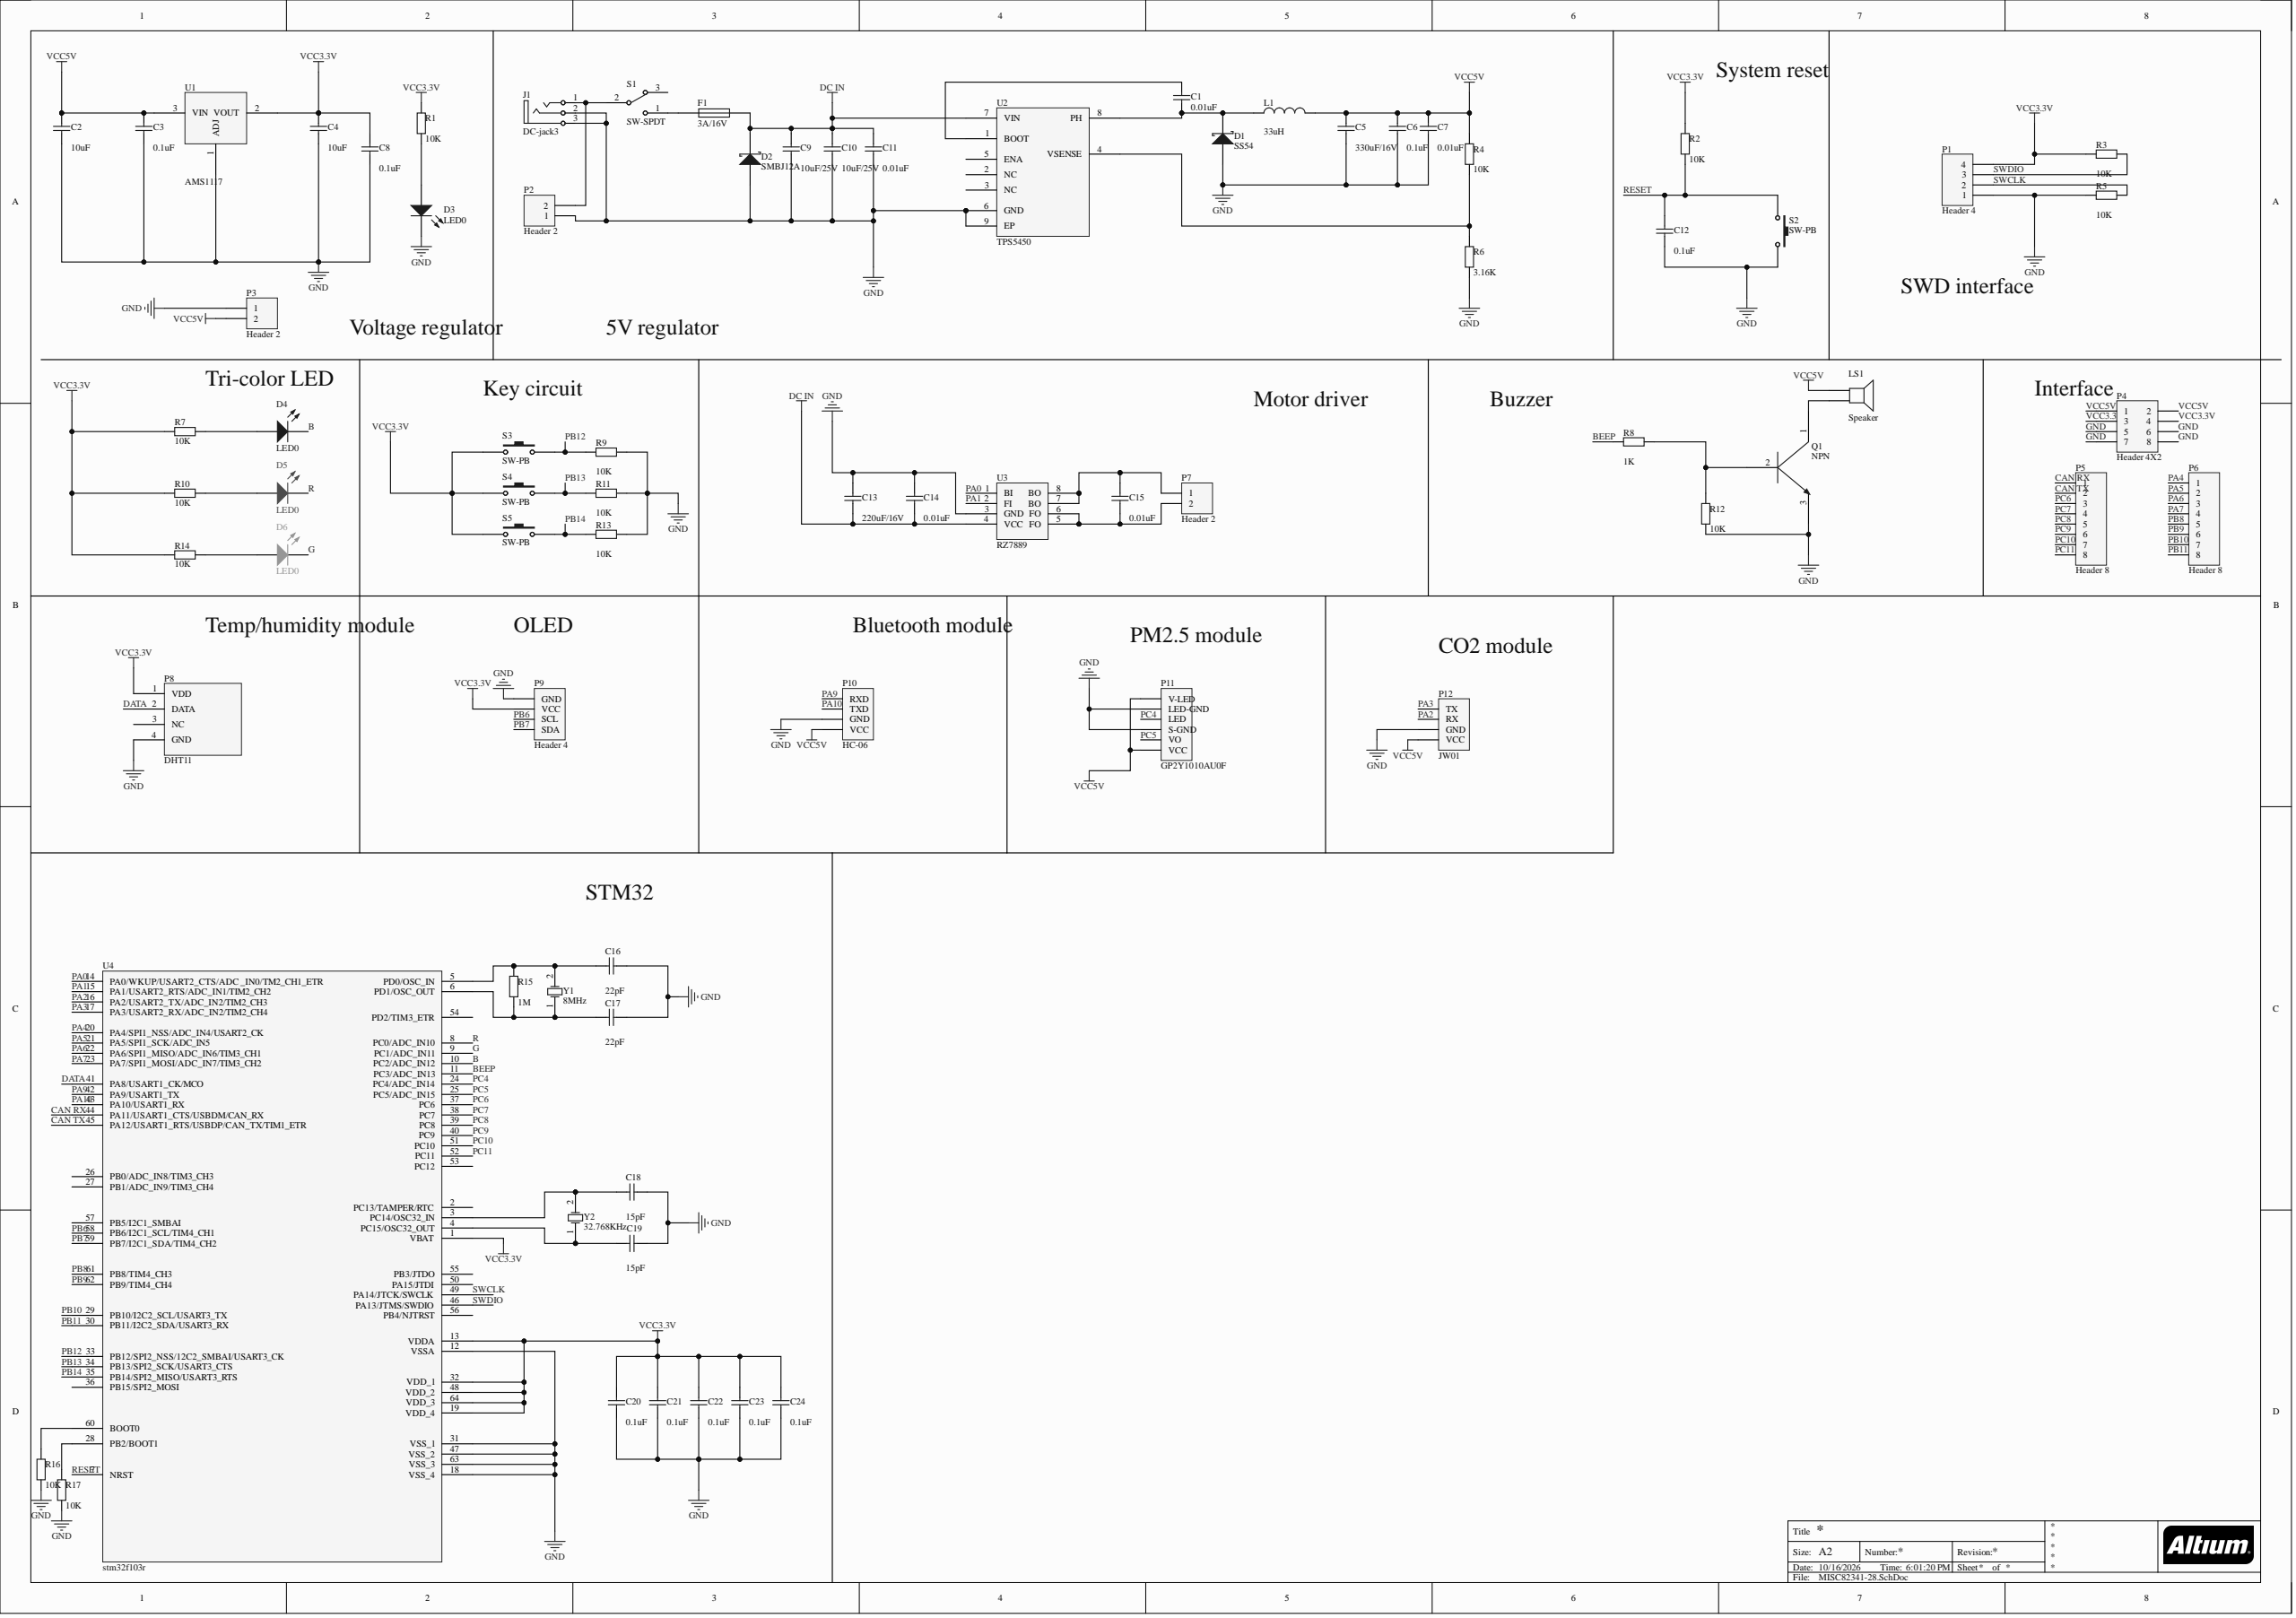Circuit board | Altium Designer | 75 parts | 60 nets
Bill of materials:
Comment,Description,Designator,Footprint,LibRef,Quantity
"0.01uF","Capacitor","C1, C7, C11, C14, C15","C0805","Cap","5"
"10uF","Capacitor","C2, C4","C0805","Cap","2"
"0.1uF","Capacitor","C3, C6, C8, C12, C20, C21, C22, C23, C24","C0805","Cap","9"
"330uF/16V","Capacitor","C5","220uF","Cap","1"
"10uF/25V","Capacitor","C9, C10","C0805","Cap","2"
"220uF/16V","Capacitor","C13","220uF","Cap","1"
"22pF","Capacitor","C16, C17","C0805","Cap","2"
"15pF","Capacitor","C18, C19","C0805","Cap","2"
"SS54","Schottky Diode","D1","SMA","D Schottky","1"
"SMBJ12A","Schottky Diode","D2","SMA","D Schottky","1"
"LED0","Typical INFRARED GaAs LED","D3, D4, D5, D6","LED0805-RD_RED","LED0","4"
"3A/16V","Fuse","F1","C70065","Fuse 1","1"
"DC-jack3","","J1","SANJIAO","DC-jack3","1"
"Inductor","Inductor","L1","DIANGAN","Inductor","1"
"Speaker","Loudspeaker","LS1","BZ","Speaker","1"
"Header 4","Header, 4-Pin","P1, P9","HDR1X4","Header 4","2"
"Header 2","Header, 2-Pin","P2, P3, P7","KF350","Header 2","3"
"Header 4X2","Header, 4-Pin, Dual row","P4","HDR2X4","Header 4X2","1"
"Header 8","Header, 8-Pin","P5, P6","HDR1X8","Header 8","2"
"DHT11","","P8","DHT11","DHT11","1"
"HC-06","Header, 4-Pin","P10","HDR1X4","Header 4","1"
"GP2Y1010AU0F","Header, 6-Pin","P11","HDR1X6","Header 6","1"
"JW01","Header, 4-Pin","P12","HDR1X4","Header 4","1"
"NPN","","Q1","QNPN","NPN","1"
"10K","Resistor","R1, R2, R3, R4, R5, R7, R9, R10, R11, R12, R13, R14, R16, R17","R0805","Res2","14"
"3.16K","Resistor","R6","R0805","Res2","1"
"1K","Resistor","R8","R0805","Res2","1"
"1M","Resistor","R15","R0805","Res2","1"
"SW-SPDT","SPDT Subminiature Toggle Switch, Right Angle Mounting, Vertical Actuation","S1","SW-TH","SW-SPDT","1"
"SW-PB","Switch","S2, S3, S4, S5","KAIGUAN","SW-PB","4"
"AMS1117","","U1","SOT-89","AMS1117","1"
"TPS5450","","U2","CYF-SOIC-H","TPS5450","1"
"RZ7889","","U3","SOP-8","RZ7889","1"
"stm32f103r","","U4","LQFP-64","stm32f103r","1"
"8MHz","Crystal Oscillator","Y1","JINGZHEN","XTAL","1"
"32.768KHz","Crystal Oscillator","Y2","R38","XTAL","1"
Netlist (Protel format):
[
C1
C0805
0.01uF



]
[
C2
C0805
10uF



]
[
C3
C0805
0.1uF



]
[
C4
C0805
10uF



]
[
C5
220uF
330uF/16V



]
[
C6
C0805
0.1uF



]
[
C7
C0805
0.01uF



]
[
C8
C0805
0.1uF



]
[
C9
C0805
10uF/25V



]
[
C10
C0805
10uF/25V



]
[
C11
C0805
0.01uF



]
[
C12
C0805
0.1uF



]
[
C13
220uF
220uF/16V



]
[
C14
C0805
0.01uF



]
[
C15
C0805
0.01uF



]
[
C16
C0805
22pF



]
[
C17
C0805
22pF



]
[
C18
C0805
15pF



]
[
C19
C0805
15pF



]
[
C20
C0805
0.1uF



]
[
C21
C0805
0.1uF



]
[
C22
C0805
0.1uF



]
[
C23
C0805
0.1uF



]
[
C24
C0805
0.1uF



]
[
D1
SMA
SS54



]
[
D2
SMA
SMBJ12A



]
[
D3
LED0805-RD_RED
LED0



]
[
D4
LED0805-RD_RED
LED0



]
[
D5
LED0805-RD_RED
LED0



]
[
D6
LED0805-RD_RED
LED0



]
[
F1
C70065
3A/16V



]
[
J1
SANJIAO
DC-jack3



]
[
L1
DIANGAN
Inductor



]
[
LS1
BZ
Speaker



]
[
P1
HDR1X4
Header 4



]
[
P2
KF350
Header 2



]
[
P3
KF350
Header 2



]
[
P4
HDR2X4
Header 4X2



]
[
P5
HDR1X8
Header 8



]
[
P6
HDR1X8
Header 8



]
[
P7
KF350
Header 2



]
[
P8
DHT11
DHT11



]
[
P9
HDR1X4
Header 4



]
[
P10
HDR1X4
HC-06



]
[
P11
HDR1X6
GP2Y1010AU0F



]
[
P12
HDR1X4
JW01



]
[
Q1
QNPN
NPN



]
[
R1
R0805
10K



]
[
R2
R0805
10K



]
[
R3
R0805
10K



]
[
R4
R0805
10K



]
[
R5
R0805
10K



]
[
R6
R0805
3.16K



]
[
R7
R0805
10K



]
[
R8
R0805
1K



]
[
R9
R0805
10K



]
[
R10
R0805
10K



]
[
R11
R0805
10K



]
[
R12
R0805
10K



]
[
R13
R0805
10K



]
[
R14
R0805
10K



]
[
R15
R0805
1M



]
[
R16
R0805
10K



]
[
R17
R0805
10K



]
[
S1
SW-TH
SW-SPDT



]
[
S2
KAIGUAN
SW-PB



]
[
S3
KAIGUAN
SW-PB



]
[
S4
KAIGUAN
SW-PB



]
[
S5
KAIGUAN
SW-PB



]
[
U1
SOT-89
AMS1117



]
[
U2
CYF-SOIC-H
TPS5450



]
[
U3
SOP-8
RZ7889



]
[
U4
LQFP-64
stm32f103r



]
[
Y1
JINGZHEN
8MHz



]
[
Y2
R38
32.768KHz



]
(
VCC5V
C2-2
C3-2
C5-2
C6-2
C7-2
L1-2
LS1-1
P3-2
P4-1
P4-2
P10-4
P11-1
P11-6
P12-4
R4-2
U1-3
)
(
VCC3.3V
C4-2
C8-2
C20-1
C21-1
C22-1
C23-1
C24-1
P1-4
P4-3
P4-4
P8-1
P9-2
R1-2
R2-2
R3-1
R7-2
R10-2
R14-2
S3-1
S4-1
S5-1
U1-2
U4-1
U4-13
U4-19
U4-32
U4-48
U4-64
)
(
SWDIO
P1-3
R3-2
U4-46
)
(
SWCLK
P1-2
R5-2
U4-49
)
(
RESET
C12-1
R2-1
S2-1
U4-7
)
(
R
D5-2
U4-8
)
(
PC11
P5-8
U4-52
)
(
PC10
P5-7
U4-51
)
(
PC9
P5-6
U4-40
)
(
PC8
P5-5
U4-39
)
(
PC7
P5-4
U4-38
)
(
PC6
P5-3
U4-37
)
(
PC5
P11-5
U4-25
)
(
PC4
P11-3
U4-24
)
(
PB14
R13-1
S5-2
U4-35
)
(
PB13
R11-1
S4-2
U4-34
)
(
PB12
R9-1
S3-2
U4-33
)
(
PB11
P6-8
U4-30
)
(
PB10
P6-7
U4-29
)
(
PB9
P6-6
U4-62
)
(
PB8
P6-5
U4-61
)
(
PB7
P9-4
U4-59
)
(
PB6
P9-3
U4-58
)
(
PA10
P10-2
U4-43
)
(
PA9
P10-1
U4-42
)
(
PA7
P6-4
U4-23
)
(
PA6
P6-3
U4-22
)
(
PA5
P6-2
U4-21
)
(
PA4
P6-1
U4-20
)
(
PA3
P12-1
U4-17
)
(
PA2
P12-2
U4-16
)
(
PA1
U3-2
U4-15
)
(
PA0
U3-1
U4-14
)
(
NetR17_2
R17-2
U4-28
)
(
NetR16_2
R16-2
U4-60
)
(
NetR4_1
R4-1
R6-2
U2-4
)
(
NetQ1_2
Q1-2
R8-2
R12-2
)
(
NetLS1_2
LS1-2
Q1-1
)
(
NetJ1_1
J1-1
P2-2
S1-2
)
(
NetF1_1
F1-1
S1-1
)
(
NetD6_1
D6-1
R14-1
)
(
NetD5_1
D5-1
R10-1
)
(
NetD4_1
D4-1
R7-1
)
(
NetD3_1
D3-1
R1-1
)
(
NetC19_1
C19-1
U4-4
Y2-1
)
(
NetC18_2
C18-2
U4-3
Y2-2
)
(
NetC17_1
C17-1
R15-1
U4-6
Y1-1
)
(
NetC16_1
C16-1
R15-2
U4-5
Y1-2
)
(
NetC15_2
C15-2
P7-1
U3-7
U3-8
)
(
NetC15_1
C15-1
P7-2
U3-5
U3-6
)
(
NetC1_2
C1-2
D1-2
L1-1
U2-8
)
(
NetC1_1
C1-1
U2-1
)
(
GND
C2-1
C3-1
C4-1
C5-1
C6-1
C7-1
C8-1
C9-1
C10-1
C11-1
C12-2
C13-2
C14-2
C16-2
C17-2
C18-1
C19-2
C20-2
C21-2
C22-2
C23-2
C24-2
D1-1
D2-1
D3-2
J1-2
J1-3
P1-1
P2-1
P3-1
P4-5
P4-6
P4-7
P4-8
P8-4
P9-1
P10-3
P11-2
P11-4
P12-3
Q1-3
R5-1
R6-1
R9-2
R11-2
R12-1
R13-2
R16-1
R17-1
S2-2
U1-1
U2-6
U2-9
U3-3
U4-12
U4-18
U4-31
U4-47
U4-63
)
(
G
D6-2
U4-9
)
(
DC IN
C9-2
C10-2
C11-2
C13-1
C14-1
D2-2
F1-2
U2-7
U3-4
)
(
DATA
P8-2
U4-41
)
(
CAN TX
P5-2
U4-45
)
(
CAN RX
P5-1
U4-44
)
(
BEEP
R8-1
U4-11
)
(
B
D4-2
U4-10
)